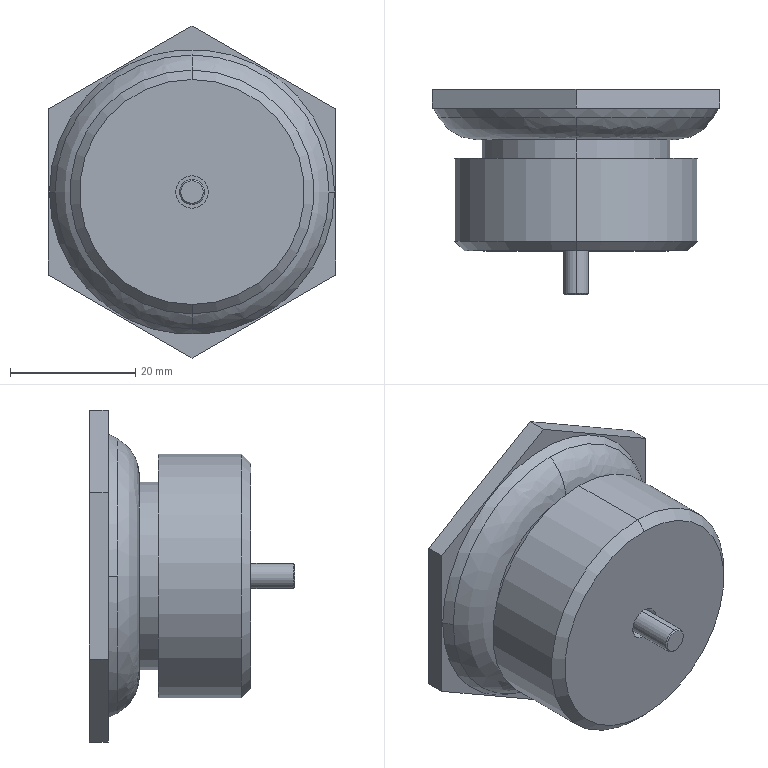Part | STEP file | _CGR01-60-U-003_1 | 1 solid | 53 faces | box 46 x 32.8 x 53.116 mm | volume 30584 mm3 | plane 29 | cylinder 14 | cone 8 | spline 2 | commonest cylinder face diameters 4 x2 5.2 x2 10 x2 10.106 x2 12 x2 30 x2